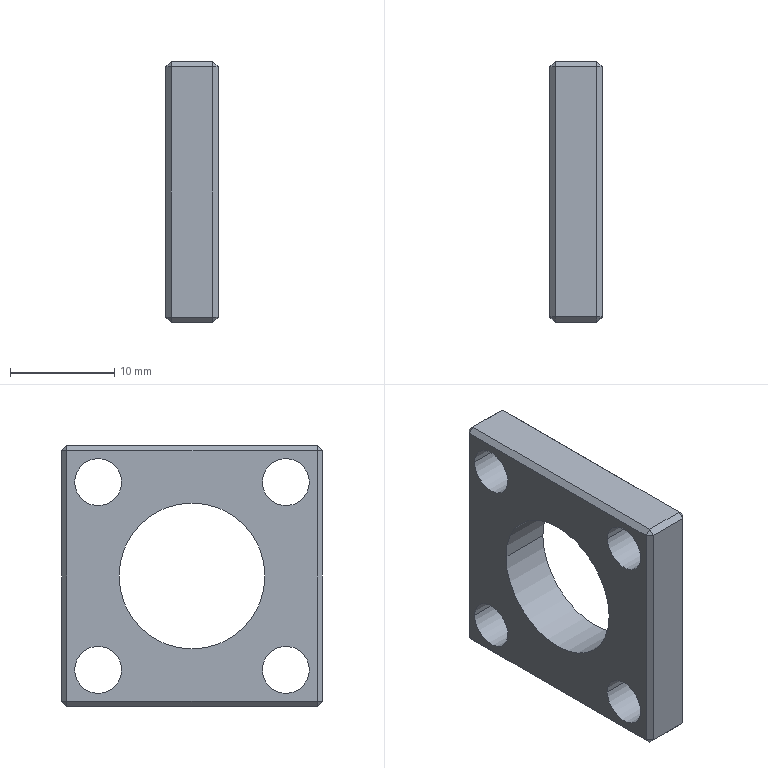Part | STEP file | 06-14 Bearing seat cover plate | 1 solid | 36 faces | box 5 x 25 x 25 mm | volume 2010 mm3 | plane 26 | cylinder 10 | commonest cylinder face diameters 4.5 x8 14 x2